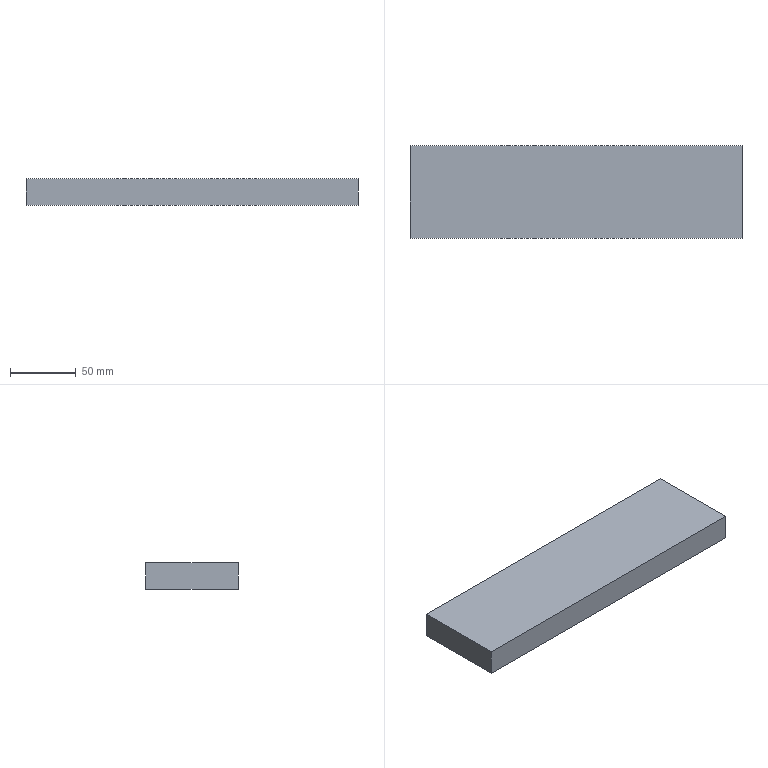Part | NX | features DATUM_CSYS 2, EXTRUDE 1, SKETCH 1 | 1 solid | 6 faces | box 252 x 70 x 20 mm | volume 352800 mm3 | plane 6
STEP:
#1=CARTESIAN_POINT('',(-126.,35.,0.));
#2=VERTEX_POINT('',#1);
#3=CARTESIAN_POINT('',(-126.,-35.,0.));
#4=VERTEX_POINT('',#3);
#5=CARTESIAN_POINT('',(-126.,35.,0.));
#6=DIRECTION('',(0.,-1.,0.));
#7=VECTOR('',#6,1000.);
#8=LINE('',#5,#7);
#9=EDGE_CURVE('',#2,#4,#8,.T.);
#10=ORIENTED_EDGE('',*,*,#9,.T.);
#11=CARTESIAN_POINT('',(-126.,-35.,20.));
#12=VERTEX_POINT('',#11);
#13=CARTESIAN_POINT('',(-126.,-35.,20.));
#14=DIRECTION('',(0.,0.,-1.));
#15=VECTOR('',#14,1000.);
#16=LINE('',#13,#15);
#17=EDGE_CURVE('',#12,#4,#16,.T.);
#18=ORIENTED_EDGE('',*,*,#17,.F.);
#19=CARTESIAN_POINT('',(-126.,35.,20.));
#20=VERTEX_POINT('',#19);
#21=CARTESIAN_POINT('',(-126.,35.,20.));
#22=DIRECTION('',(0.,-1.,0.));
#23=VECTOR('',#22,1000.);
#24=LINE('',#21,#23);
#25=EDGE_CURVE('',#20,#12,#24,.T.);
#26=ORIENTED_EDGE('',*,*,#25,.F.);
#27=CARTESIAN_POINT('',(-126.,35.,20.));
#28=DIRECTION('',(0.,0.,-1.));
#29=VECTOR('',#28,1000.);
#30=LINE('',#27,#29);
#31=EDGE_CURVE('',#20,#2,#30,.T.);
#32=ORIENTED_EDGE('',*,*,#31,.T.);
#33=EDGE_LOOP('',(#10,#18,#26,#32));
#34=FACE_BOUND('',#33,.T.);
#35=CARTESIAN_POINT('',(-126.,35.,20.));
#36=DIRECTION('',(1.,0.,0.));
#37=DIRECTION('',(0.,0.,-1.));
#38=AXIS2_PLACEMENT_3D('',#35,#36,#37);
#39=PLANE('',#38);
#40=ADVANCED_FACE('',(#34),#39,.F.);
#41=CARTESIAN_POINT('',(126.,-35.,0.));
#42=VERTEX_POINT('',#41);
#43=CARTESIAN_POINT('',(-126.,-35.,0.));
#44=DIRECTION('',(1.,0.,0.));
#45=VECTOR('',#44,1000.);
#46=LINE('',#43,#45);
#47=EDGE_CURVE('',#4,#42,#46,.T.);
#48=ORIENTED_EDGE('',*,*,#47,.T.);
#49=CARTESIAN_POINT('',(126.,-35.,20.));
#50=VERTEX_POINT('',#49);
#51=CARTESIAN_POINT('',(126.,-35.,20.));
#52=DIRECTION('',(0.,0.,-1.));
#53=VECTOR('',#52,1000.);
#54=LINE('',#51,#53);
#55=EDGE_CURVE('',#50,#42,#54,.T.);
#56=ORIENTED_EDGE('',*,*,#55,.F.);
#57=CARTESIAN_POINT('',(-126.,-35.,20.));
#58=DIRECTION('',(1.,0.,0.));
#59=VECTOR('',#58,1000.);
#60=LINE('',#57,#59);
#61=EDGE_CURVE('',#12,#50,#60,.T.);
#62=ORIENTED_EDGE('',*,*,#61,.F.);
#63=ORIENTED_EDGE('',*,*,#17,.T.);
#64=EDGE_LOOP('',(#48,#56,#62,#63));
#65=FACE_BOUND('',#64,.T.);
#66=CARTESIAN_POINT('',(-126.,-35.,20.));
#67=DIRECTION('',(0.,1.,0.));
#68=DIRECTION('',(0.,0.,1.));
#69=AXIS2_PLACEMENT_3D('',#66,#67,#68);
#70=PLANE('',#69);
#71=ADVANCED_FACE('',(#65),#70,.F.);
#72=CARTESIAN_POINT('',(126.,35.,0.));
#73=VERTEX_POINT('',#72);
#74=CARTESIAN_POINT('',(126.,-35.,0.));
#75=DIRECTION('',(0.,1.,0.));
#76=VECTOR('',#75,1000.);
#77=LINE('',#74,#76);
#78=EDGE_CURVE('',#42,#73,#77,.T.);
#79=ORIENTED_EDGE('',*,*,#78,.T.);
#80=CARTESIAN_POINT('',(126.,35.,20.));
#81=VERTEX_POINT('',#80);
#82=CARTESIAN_POINT('',(126.,35.,20.));
#83=DIRECTION('',(0.,0.,-1.));
#84=VECTOR('',#83,1000.);
#85=LINE('',#82,#84);
#86=EDGE_CURVE('',#81,#73,#85,.T.);
#87=ORIENTED_EDGE('',*,*,#86,.F.);
#88=CARTESIAN_POINT('',(126.,-35.,20.));
#89=DIRECTION('',(0.,1.,0.));
#90=VECTOR('',#89,1000.);
#91=LINE('',#88,#90);
#92=EDGE_CURVE('',#50,#81,#91,.T.);
#93=ORIENTED_EDGE('',*,*,#92,.F.);
#94=ORIENTED_EDGE('',*,*,#55,.T.);
#95=EDGE_LOOP('',(#79,#87,#93,#94));
#96=FACE_BOUND('',#95,.T.);
#97=CARTESIAN_POINT('',(126.,-35.,20.));
#98=DIRECTION('',(-1.,0.,0.));
#99=DIRECTION('',(0.,0.,1.));
#100=AXIS2_PLACEMENT_3D('',#97,#98,#99);
#101=PLANE('',#100);
#102=ADVANCED_FACE('',(#96),#101,.F.);
#103=CARTESIAN_POINT('',(126.,35.,0.));
#104=DIRECTION('',(-1.,0.,0.));
#105=VECTOR('',#104,1000.);
#106=LINE('',#103,#105);
#107=EDGE_CURVE('',#73,#2,#106,.T.);
#108=ORIENTED_EDGE('',*,*,#107,.T.);
#109=ORIENTED_EDGE('',*,*,#31,.F.);
#110=CARTESIAN_POINT('',(126.,35.,20.));
#111=DIRECTION('',(-1.,0.,0.));
#112=VECTOR('',#111,1000.);
#113=LINE('',#110,#112);
#114=EDGE_CURVE('',#81,#20,#113,.T.);
#115=ORIENTED_EDGE('',*,*,#114,.F.);
#116=ORIENTED_EDGE('',*,*,#86,.T.);
#117=EDGE_LOOP('',(#108,#109,#115,#116));
#118=FACE_BOUND('',#117,.T.);
#119=CARTESIAN_POINT('',(126.,35.,20.));
#120=DIRECTION('',(0.,-1.,0.));
#121=DIRECTION('',(0.,0.,-1.));
#122=AXIS2_PLACEMENT_3D('',#119,#120,#121);
#123=PLANE('',#122);
#124=ADVANCED_FACE('',(#118),#123,.F.);
#125=ORIENTED_EDGE('',*,*,#25,.T.);
#126=ORIENTED_EDGE('',*,*,#61,.T.);
#127=ORIENTED_EDGE('',*,*,#92,.T.);
#128=ORIENTED_EDGE('',*,*,#114,.T.);
#129=EDGE_LOOP('',(#125,#126,#127,#128));
#130=FACE_BOUND('',#129,.T.);
#131=CARTESIAN_POINT('',(0.,0.,20.));
#132=DIRECTION('',(0.,0.,1.));
#133=DIRECTION('',(1.,0.,0.));
#134=AXIS2_PLACEMENT_3D('',#131,#132,#133);
#135=PLANE('',#134);
#136=ADVANCED_FACE('',(#130),#135,.T.);
#137=ORIENTED_EDGE('',*,*,#9,.F.);
#138=ORIENTED_EDGE('',*,*,#107,.F.);
#139=ORIENTED_EDGE('',*,*,#78,.F.);
#140=ORIENTED_EDGE('',*,*,#47,.F.);
#141=EDGE_LOOP('',(#137,#138,#139,#140));
#142=FACE_BOUND('',#141,.T.);
#143=CARTESIAN_POINT('',(0.,0.,0.));
#144=DIRECTION('',(0.,0.,1.));
#145=DIRECTION('',(1.,0.,0.));
#146=AXIS2_PLACEMENT_3D('',#143,#144,#145);
#147=PLANE('',#146);
#148=ADVANCED_FACE('',(#142),#147,.F.);
#149=CLOSED_SHELL('',(#40,#71,#102,#124,#136,#148));
#150=MANIFOLD_SOLID_BREP('',#149);
#151=(LENGTH_UNIT()NAMED_UNIT(*)SI_UNIT(.MILLI.,.METRE.));
#152=UNCERTAINTY_MEASURE_WITH_UNIT(LENGTH_MEASURE(0.00001),#151,'','');
#153=(NAMED_UNIT(*)PLANE_ANGLE_UNIT()SI_UNIT($,.RADIAN.));
#154=(NAMED_UNIT(*)SI_UNIT($,.STERADIAN.)SOLID_ANGLE_UNIT());
#155=(GEOMETRIC_REPRESENTATION_CONTEXT(3)GLOBAL_UNCERTAINTY_ASSIGNED_CONTEXT((#152))GLOBAL_UNIT_ASSIGNED_CONTEXT((#151,#153,#154))REPRESENTATION_CONTEXT('',''));
#156=ADVANCED_BREP_SHAPE_REPRESENTATION('',(#150),#155);